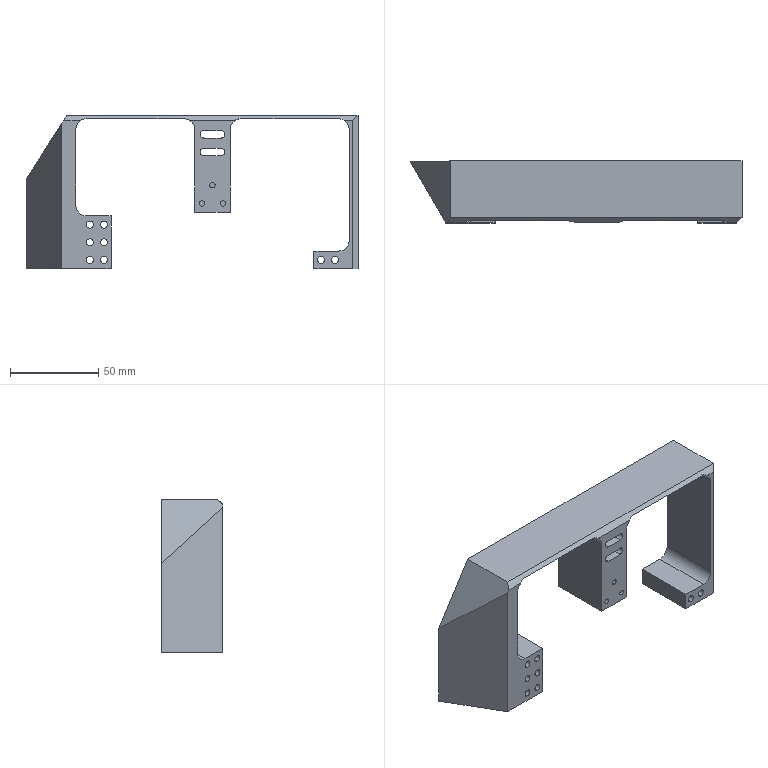Part | SolidWorks | features ICE 9, Fillet 4, MirrorPattern 3, Chamfer 1, Extrusion 1, LPattern 1 | 1 solid | 71 faces | box 188.207 x 35 x 87 mm | volume 133401 mm3 | cylinder 38 | plane 33 | commonest cylinder face diameters 4 x16 3 x12 12 x6 4.24 x4